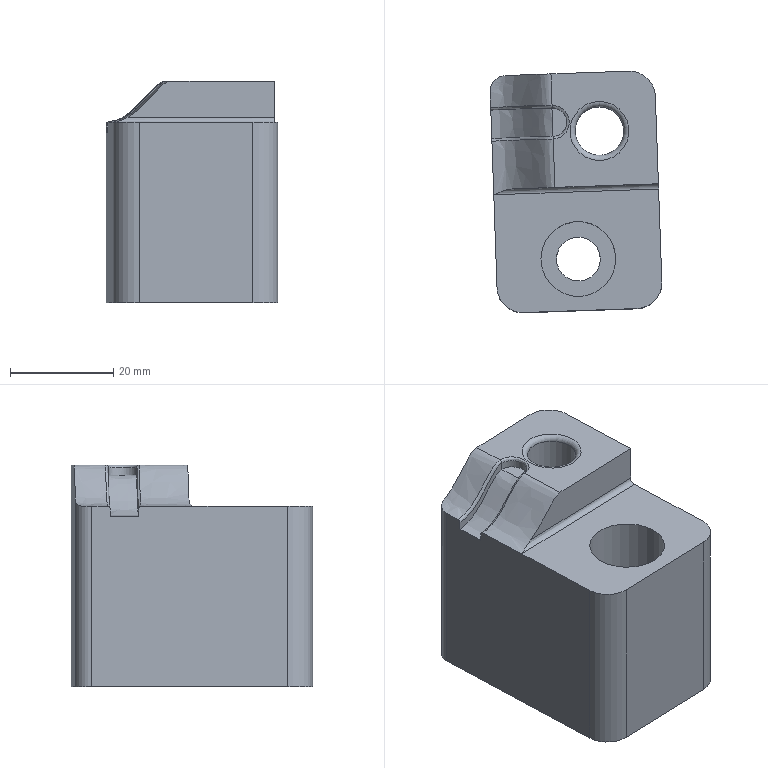Part | NX | features DIE-62 2 | 1 solid | 28 faces | box 33.258 x 46.744 x 43 mm | volume 48412 mm3 | plane 10 | spline 9 | cylinder 8 | torus 1 | commonest cylinder face diameters 10 x3 2 x1 6 x1 8.5 x1 9.44 x1 14.5 x1